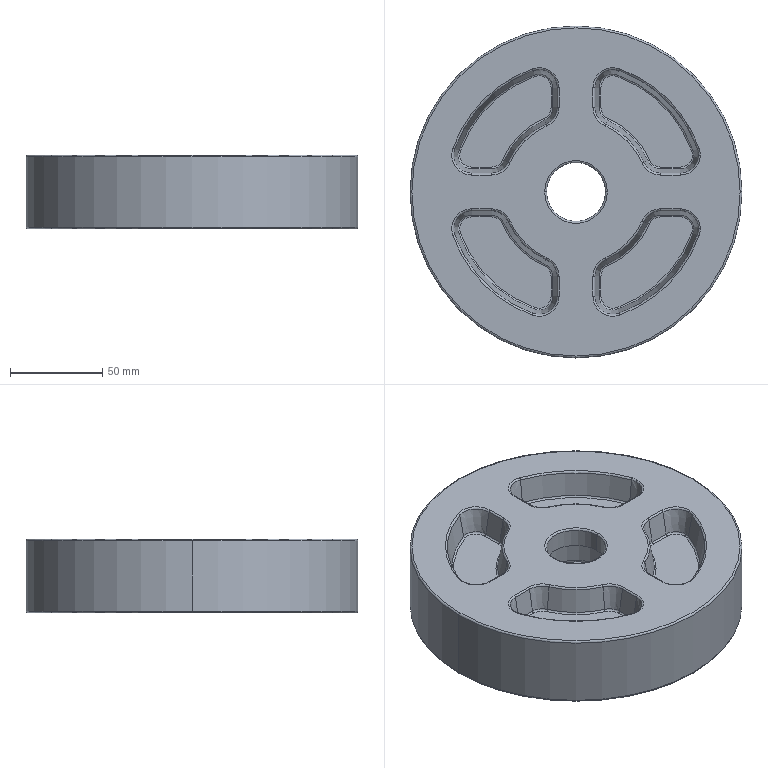Part | SolidWorks | features ICE 7, Fillet 2, CirPattern 1, Extrusion 1, MirrorPattern 1 | 1 solid | 243 faces | box 180 x 180 x 40 mm | volume 747348 mm3 | torus 112 | cylinder 50 | cone 48 | plane 33 | commonest cylinder face diameters 2 x32 3 x6 52 x4 32 x2 45 x2 55 x2